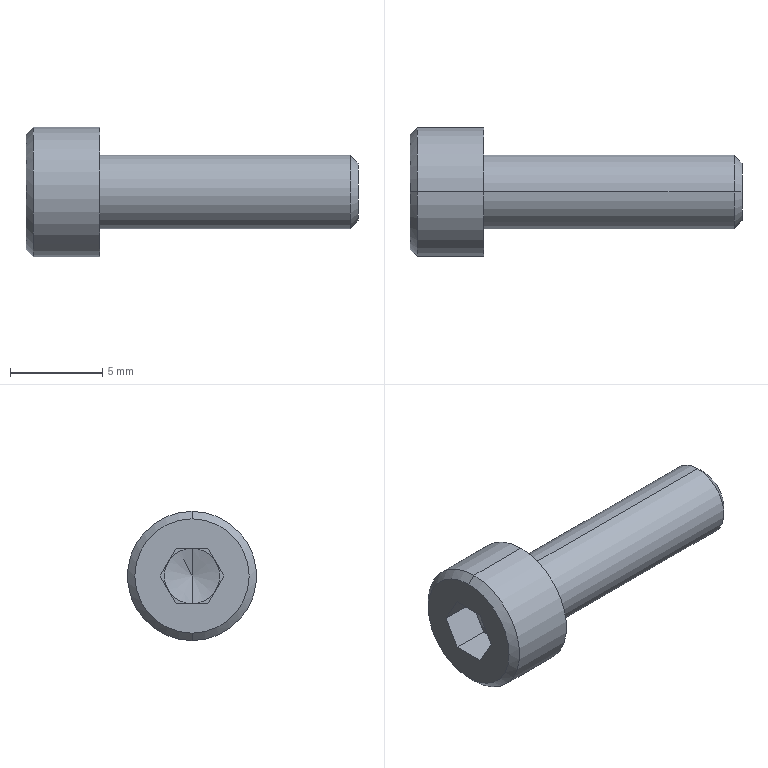Part | SolidWorks | features BaseBody 1 | 1 solid | 25 faces | box 18 x 7 x 7 mm | volume 310.563 mm3 | plane 15 | cone 6 | cylinder 4 | commonest cylinder face diameters 4 x2 7 x2
STEP:
#1=CARTESIAN_POINT('',(-4.,0.,3.1));
#2=VERTEX_POINT('',#1);
#3=CARTESIAN_POINT('',(-4.,0.,-3.1));
#4=VERTEX_POINT('',#3);
#5=CARTESIAN_POINT('',(-4.,0.,0.));
#6=DIRECTION('',(1.,0.,0.));
#7=DIRECTION('',(0.,0.,-1.));
#8=AXIS2_PLACEMENT_3D('',#5,#6,#7);
#9=CIRCLE('',#8,3.1);
#10=EDGE_CURVE('',#2,#4,#9,.T.);
#11=ORIENTED_EDGE('',*,*,#10,.F.);
#12=CARTESIAN_POINT('',(-4.,0.,0.));
#13=DIRECTION('',(1.,0.,0.));
#14=DIRECTION('',(0.,0.,-1.));
#15=AXIS2_PLACEMENT_3D('',#12,#13,#14);
#16=CIRCLE('',#15,3.1);
#17=EDGE_CURVE('',#4,#2,#16,.T.);
#18=ORIENTED_EDGE('',*,*,#17,.F.);
#19=EDGE_LOOP('',(#11,#18));
#20=FACE_OUTER_BOUND('',#19,.T.);
#21=CARTESIAN_POINT('',(-4.,-1.732,0.));
#22=VERTEX_POINT('',#21);
#23=CARTESIAN_POINT('',(-4.,-0.866,-1.5));
#24=VERTEX_POINT('',#23);
#25=CARTESIAN_POINT('',(-4.,-1.732,0.));
#26=DIRECTION('',(0.,0.5,-0.866));
#27=VECTOR('',#26,1000.);
#28=LINE('',#25,#27);
#29=EDGE_CURVE('',#22,#24,#28,.T.);
#30=ORIENTED_EDGE('',*,*,#29,.T.);
#31=CARTESIAN_POINT('',(-4.,0.866,-1.5));
#32=VERTEX_POINT('',#31);
#33=CARTESIAN_POINT('',(-4.,-0.866,-1.5));
#34=DIRECTION('',(0.,1.,0.));
#35=VECTOR('',#34,1000.);
#36=LINE('',#33,#35);
#37=EDGE_CURVE('',#24,#32,#36,.T.);
#38=ORIENTED_EDGE('',*,*,#37,.T.);
#39=CARTESIAN_POINT('',(-4.,1.732,0.));
#40=VERTEX_POINT('',#39);
#41=CARTESIAN_POINT('',(-4.,0.866,-1.5));
#42=DIRECTION('',(0.,0.5,0.866));
#43=VECTOR('',#42,1000.);
#44=LINE('',#41,#43);
#45=EDGE_CURVE('',#32,#40,#44,.T.);
#46=ORIENTED_EDGE('',*,*,#45,.T.);
#47=CARTESIAN_POINT('',(-4.,0.866,1.5));
#48=VERTEX_POINT('',#47);
#49=CARTESIAN_POINT('',(-4.,1.732,0.));
#50=DIRECTION('',(0.,-0.5,0.866));
#51=VECTOR('',#50,1000.);
#52=LINE('',#49,#51);
#53=EDGE_CURVE('',#40,#48,#52,.T.);
#54=ORIENTED_EDGE('',*,*,#53,.T.);
#55=CARTESIAN_POINT('',(-4.,-0.866,1.5));
#56=VERTEX_POINT('',#55);
#57=CARTESIAN_POINT('',(-4.,0.866,1.5));
#58=DIRECTION('',(0.,-1.,0.));
#59=VECTOR('',#58,1000.);
#60=LINE('',#57,#59);
#61=EDGE_CURVE('',#48,#56,#60,.T.);
#62=ORIENTED_EDGE('',*,*,#61,.T.);
#63=CARTESIAN_POINT('',(-4.,-0.866,1.5));
#64=DIRECTION('',(0.,-0.5,-0.866));
#65=VECTOR('',#64,1000.);
#66=LINE('',#63,#65);
#67=EDGE_CURVE('',#56,#22,#66,.T.);
#68=ORIENTED_EDGE('',*,*,#67,.T.);
#69=EDGE_LOOP('',(#30,#38,#46,#54,#62,#68));
#70=FACE_BOUND('',#69,.T.);
#71=CARTESIAN_POINT('',(-4.,0.,0.));
#72=DIRECTION('',(1.,0.,0.));
#73=DIRECTION('',(0.,0.,-1.));
#74=AXIS2_PLACEMENT_3D('',#71,#72,#73);
#75=PLANE('',#74);
#76=ADVANCED_FACE('',(#20,#70),#75,.F.);
#77=ORIENTED_EDGE('',*,*,#67,.F.);
#78=CARTESIAN_POINT('',(-2.,-0.866,1.5));
#79=VERTEX_POINT('',#78);
#80=CARTESIAN_POINT('',(-2.,-0.866,1.5));
#81=DIRECTION('',(-1.,0.,0.));
#82=VECTOR('',#81,1000.);
#83=LINE('',#80,#82);
#84=EDGE_CURVE('',#79,#56,#83,.T.);
#85=ORIENTED_EDGE('',*,*,#84,.F.);
#86=CARTESIAN_POINT('',(-2.,-1.299,0.75));
#87=VERTEX_POINT('',#86);
#88=CARTESIAN_POINT('',(-2.,-0.866,1.5));
#89=DIRECTION('',(0.,-0.5,-0.866));
#90=VECTOR('',#89,1000.);
#91=LINE('',#88,#90);
#92=EDGE_CURVE('',#79,#87,#91,.T.);
#93=ORIENTED_EDGE('',*,*,#92,.T.);
#94=CARTESIAN_POINT('',(-2.,-1.732,0.));
#95=VERTEX_POINT('',#94);
#96=CARTESIAN_POINT('',(-2.,-0.866,1.5));
#97=DIRECTION('',(0.,-0.5,-0.866));
#98=VECTOR('',#97,1000.);
#99=LINE('',#96,#98);
#100=EDGE_CURVE('',#87,#95,#99,.T.);
#101=ORIENTED_EDGE('',*,*,#100,.T.);
#102=CARTESIAN_POINT('',(-2.,-1.732,0.));
#103=DIRECTION('',(-1.,0.,0.));
#104=VECTOR('',#103,1000.);
#105=LINE('',#102,#104);
#106=EDGE_CURVE('',#95,#22,#105,.T.);
#107=ORIENTED_EDGE('',*,*,#106,.T.);
#108=EDGE_LOOP('',(#77,#85,#93,#101,#107));
#109=FACE_OUTER_BOUND('',#108,.T.);
#110=CARTESIAN_POINT('',(-2.,-0.866,1.5));
#111=DIRECTION('',(0.,0.866,-0.5));
#112=DIRECTION('',(0.,0.5,0.866));
#113=AXIS2_PLACEMENT_3D('',#110,#111,#112);
#114=PLANE('',#113);
#115=ADVANCED_FACE('',(#109),#114,.T.);
#116=ORIENTED_EDGE('',*,*,#29,.F.);
#117=ORIENTED_EDGE('',*,*,#106,.F.);
#118=CARTESIAN_POINT('',(-2.,-1.299,-0.75));
#119=VERTEX_POINT('',#118);
#120=CARTESIAN_POINT('',(-2.,-1.732,0.));
#121=DIRECTION('',(0.,0.5,-0.866));
#122=VECTOR('',#121,1000.);
#123=LINE('',#120,#122);
#124=EDGE_CURVE('',#95,#119,#123,.T.);
#125=ORIENTED_EDGE('',*,*,#124,.T.);
#126=CARTESIAN_POINT('',(-2.,-0.866,-1.5));
#127=VERTEX_POINT('',#126);
#128=CARTESIAN_POINT('',(-2.,-1.732,0.));
#129=DIRECTION('',(0.,0.5,-0.866));
#130=VECTOR('',#129,1000.);
#131=LINE('',#128,#130);
#132=EDGE_CURVE('',#119,#127,#131,.T.);
#133=ORIENTED_EDGE('',*,*,#132,.T.);
#134=CARTESIAN_POINT('',(-2.,-0.866,-1.5));
#135=DIRECTION('',(-1.,0.,0.));
#136=VECTOR('',#135,1000.);
#137=LINE('',#134,#136);
#138=EDGE_CURVE('',#127,#24,#137,.T.);
#139=ORIENTED_EDGE('',*,*,#138,.T.);
#140=EDGE_LOOP('',(#116,#117,#125,#133,#139));
#141=FACE_OUTER_BOUND('',#140,.T.);
#142=CARTESIAN_POINT('',(-2.,-1.732,0.));
#143=DIRECTION('',(0.,0.866,0.5));
#144=DIRECTION('',(0.,-0.5,0.866));
#145=AXIS2_PLACEMENT_3D('',#142,#143,#144);
#146=PLANE('',#145);
#147=ADVANCED_FACE('',(#141),#146,.T.);
#148=ORIENTED_EDGE('',*,*,#37,.F.);
#149=ORIENTED_EDGE('',*,*,#138,.F.);
#150=CARTESIAN_POINT('',(-2.,0.,-1.5));
#151=VERTEX_POINT('',#150);
#152=CARTESIAN_POINT('',(-2.,-0.866,-1.5));
#153=DIRECTION('',(0.,1.,0.));
#154=VECTOR('',#153,1000.);
#155=LINE('',#152,#154);
#156=EDGE_CURVE('',#127,#151,#155,.T.);
#157=ORIENTED_EDGE('',*,*,#156,.T.);
#158=CARTESIAN_POINT('',(-2.,0.866,-1.5));
#159=VERTEX_POINT('',#158);
#160=CARTESIAN_POINT('',(-2.,-0.866,-1.5));
#161=DIRECTION('',(0.,1.,0.));
#162=VECTOR('',#161,1000.);
#163=LINE('',#160,#162);
#164=EDGE_CURVE('',#151,#159,#163,.T.);
#165=ORIENTED_EDGE('',*,*,#164,.T.);
#166=CARTESIAN_POINT('',(-2.,0.866,-1.5));
#167=DIRECTION('',(-1.,0.,0.));
#168=VECTOR('',#167,1000.);
#169=LINE('',#166,#168);
#170=EDGE_CURVE('',#159,#32,#169,.T.);
#171=ORIENTED_EDGE('',*,*,#170,.T.);
#172=EDGE_LOOP('',(#148,#149,#157,#165,#171));
#173=FACE_OUTER_BOUND('',#172,.T.);
#174=CARTESIAN_POINT('',(-2.,-0.866,-1.5));
#175=DIRECTION('',(0.,0.,1.));
#176=DIRECTION('',(1.,0.,0.));
#177=AXIS2_PLACEMENT_3D('',#174,#175,#176);
#178=PLANE('',#177);
#179=ADVANCED_FACE('',(#173),#178,.T.);
#180=ORIENTED_EDGE('',*,*,#45,.F.);
#181=ORIENTED_EDGE('',*,*,#170,.F.);
#182=CARTESIAN_POINT('',(-2.,1.299,-0.75));
#183=VERTEX_POINT('',#182);
#184=CARTESIAN_POINT('',(-2.,0.866,-1.5));
#185=DIRECTION('',(0.,0.5,0.866));
#186=VECTOR('',#185,1000.);
#187=LINE('',#184,#186);
#188=EDGE_CURVE('',#159,#183,#187,.T.);
#189=ORIENTED_EDGE('',*,*,#188,.T.);
#190=CARTESIAN_POINT('',(-2.,1.732,0.));
#191=VERTEX_POINT('',#190);
#192=CARTESIAN_POINT('',(-2.,0.866,-1.5));
#193=DIRECTION('',(0.,0.5,0.866));
#194=VECTOR('',#193,1000.);
#195=LINE('',#192,#194);
#196=EDGE_CURVE('',#183,#191,#195,.T.);
#197=ORIENTED_EDGE('',*,*,#196,.T.);
#198=CARTESIAN_POINT('',(-2.,1.732,0.));
#199=DIRECTION('',(-1.,0.,0.));
#200=VECTOR('',#199,1000.);
#201=LINE('',#198,#200);
#202=EDGE_CURVE('',#191,#40,#201,.T.);
#203=ORIENTED_EDGE('',*,*,#202,.T.);
#204=EDGE_LOOP('',(#180,#181,#189,#197,#203));
#205=FACE_OUTER_BOUND('',#204,.T.);
#206=CARTESIAN_POINT('',(-2.,0.866,-1.5));
#207=DIRECTION('',(0.,-0.866,0.5));
#208=DIRECTION('',(0.,-0.5,-0.866));
#209=AXIS2_PLACEMENT_3D('',#206,#207,#208);
#210=PLANE('',#209);
#211=ADVANCED_FACE('',(#205),#210,.T.);
#212=ORIENTED_EDGE('',*,*,#53,.F.);
#213=ORIENTED_EDGE('',*,*,#202,.F.);
#214=CARTESIAN_POINT('',(-2.,1.299,0.75));
#215=VERTEX_POINT('',#214);
#216=CARTESIAN_POINT('',(-2.,1.732,0.));
#217=DIRECTION('',(0.,-0.5,0.866));
#218=VECTOR('',#217,1000.);
#219=LINE('',#216,#218);
#220=EDGE_CURVE('',#191,#215,#219,.T.);
#221=ORIENTED_EDGE('',*,*,#220,.T.);
#222=CARTESIAN_POINT('',(-2.,0.866,1.5));
#223=VERTEX_POINT('',#222);
#224=CARTESIAN_POINT('',(-2.,1.732,0.));
#225=DIRECTION('',(0.,-0.5,0.866));
#226=VECTOR('',#225,1000.);
#227=LINE('',#224,#226);
#228=EDGE_CURVE('',#215,#223,#227,.T.);
#229=ORIENTED_EDGE('',*,*,#228,.T.);
#230=CARTESIAN_POINT('',(-2.,0.866,1.5));
#231=DIRECTION('',(-1.,0.,0.));
#232=VECTOR('',#231,1000.);
#233=LINE('',#230,#232);
#234=EDGE_CURVE('',#223,#48,#233,.T.);
#235=ORIENTED_EDGE('',*,*,#234,.T.);
#236=EDGE_LOOP('',(#212,#213,#221,#229,#235));
#237=FACE_OUTER_BOUND('',#236,.T.);
#238=CARTESIAN_POINT('',(-2.,1.732,0.));
#239=DIRECTION('',(0.,-0.866,-0.5));
#240=DIRECTION('',(0.,0.5,-0.866));
#241=AXIS2_PLACEMENT_3D('',#238,#239,#240);
#242=PLANE('',#241);
#243=ADVANCED_FACE('',(#237),#242,.T.);
#244=ORIENTED_EDGE('',*,*,#61,.F.);
#245=ORIENTED_EDGE('',*,*,#234,.F.);
#246=CARTESIAN_POINT('',(-2.,0.,1.5));
#247=VERTEX_POINT('',#246);
#248=CARTESIAN_POINT('',(-2.,0.866,1.5));
#249=DIRECTION('',(0.,-1.,0.));
#250=VECTOR('',#249,1000.);
#251=LINE('',#248,#250);
#252=EDGE_CURVE('',#223,#247,#251,.T.);
#253=ORIENTED_EDGE('',*,*,#252,.T.);
#254=CARTESIAN_POINT('',(-2.,0.866,1.5));
#255=DIRECTION('',(0.,-1.,0.));
#256=VECTOR('',#255,1000.);
#257=LINE('',#254,#256);
#258=EDGE_CURVE('',#247,#79,#257,.T.);
#259=ORIENTED_EDGE('',*,*,#258,.T.);
#260=ORIENTED_EDGE('',*,*,#84,.T.);
#261=EDGE_LOOP('',(#244,#245,#253,#259,#260));
#262=FACE_OUTER_BOUND('',#261,.T.);
#263=CARTESIAN_POINT('',(-2.,0.866,1.5));
#264=DIRECTION('',(0.,0.,-1.));
#265=DIRECTION('',(-1.,0.,0.));
#266=AXIS2_PLACEMENT_3D('',#263,#264,#265);
#267=PLANE('',#266);
#268=ADVANCED_FACE('',(#262),#267,.T.);
#269=CARTESIAN_POINT('',(-2.,0.,0.));
#270=DIRECTION('',(1.,0.,0.));
#271=DIRECTION('',(0.,0.,-1.));
#272=AXIS2_PLACEMENT_3D('',#269,#270,#271);
#273=CIRCLE('',#272,1.5);
#274=EDGE_CURVE('',#247,#87,#273,.T.);
#275=ORIENTED_EDGE('',*,*,#274,.T.);
#276=ORIENTED_EDGE('',*,*,#92,.F.);
#277=ORIENTED_EDGE('',*,*,#258,.F.);
#278=EDGE_LOOP('',(#275,#276,#277));
#279=FACE_OUTER_BOUND('',#278,.T.);
#280=CARTESIAN_POINT('',(-2.,0.,0.));
#281=DIRECTION('',(1.,0.,0.));
#282=DIRECTION('',(0.,0.,-1.));
#283=AXIS2_PLACEMENT_3D('',#280,#281,#282);
#284=PLANE('',#283);
#285=ADVANCED_FACE('',(#279),#284,.F.);
#286=CARTESIAN_POINT('',(-1.598,0.,0.));
#287=VERTEX_POINT('',#286);
#288=CARTESIAN_POINT('',(-1.598,0.,0.));
#289=DIRECTION('',(-0.2588,0.,-0.9659));
#290=VECTOR('',#289,1000.);
#291=LINE('',#288,#290);
#292=EDGE_CURVE('',#287,#151,#291,.T.);
#293=ORIENTED_EDGE('',*,*,#292,.T.);
#294=CARTESIAN_POINT('',(-2.,0.,0.));
#295=DIRECTION('',(1.,0.,0.));
#296=DIRECTION('',(0.,0.,-1.));
#297=AXIS2_PLACEMENT_3D('',#294,#295,#296);
#298=CIRCLE('',#297,1.5);
#299=EDGE_CURVE('',#119,#151,#298,.T.);
#300=ORIENTED_EDGE('',*,*,#299,.F.);
#301=CARTESIAN_POINT('',(-2.,0.,0.));
#302=DIRECTION('',(1.,0.,0.));
#303=DIRECTION('',(0.,0.,-1.));
#304=AXIS2_PLACEMENT_3D('',#301,#302,#303);
#305=CIRCLE('',#304,1.5);
#306=EDGE_CURVE('',#87,#119,#305,.T.);
#307=ORIENTED_EDGE('',*,*,#306,.F.);
#308=ORIENTED_EDGE('',*,*,#274,.F.);
#309=CARTESIAN_POINT('',(-1.598,0.,0.));
#310=DIRECTION('',(-0.2588,0.,0.9659));
#311=VECTOR('',#310,1000.);
#312=LINE('',#309,#311);
#313=EDGE_CURVE('',#287,#247,#312,.T.);
#314=ORIENTED_EDGE('',*,*,#313,.F.);
#315=EDGE_LOOP('',(#293,#300,#307,#308,#314));
#316=FACE_OUTER_BOUND('',#315,.T.);
#317=CARTESIAN_POINT('',(-2.,0.,0.));
#318=DIRECTION('',(-1.,0.,0.));
#319=DIRECTION('',(0.,1.,0.));
#320=AXIS2_PLACEMENT_3D('',#317,#318,#319);
#321=CONICAL_SURFACE('',#320,1.5,1.309);
#322=ADVANCED_FACE('',(#316),#321,.F.);
#323=ORIENTED_EDGE('',*,*,#313,.T.);
#324=CARTESIAN_POINT('',(-2.,0.,0.));
#325=DIRECTION('',(1.,0.,0.));
#326=DIRECTION('',(0.,0.,-1.));
#327=AXIS2_PLACEMENT_3D('',#324,#325,#326);
#328=CIRCLE('',#327,1.5);
#329=EDGE_CURVE('',#215,#247,#328,.T.);
#330=ORIENTED_EDGE('',*,*,#329,.F.);
#331=CARTESIAN_POINT('',(-2.,0.,0.));
#332=DIRECTION('',(1.,0.,0.));
#333=DIRECTION('',(0.,0.,-1.));
#334=AXIS2_PLACEMENT_3D('',#331,#332,#333);
#335=CIRCLE('',#334,1.5);
#336=EDGE_CURVE('',#183,#215,#335,.T.);
#337=ORIENTED_EDGE('',*,*,#336,.F.);
#338=CARTESIAN_POINT('',(-2.,0.,0.));
#339=DIRECTION('',(1.,0.,0.));
#340=DIRECTION('',(0.,0.,-1.));
#341=AXIS2_PLACEMENT_3D('',#338,#339,#340);
#342=CIRCLE('',#341,1.5);
#343=EDGE_CURVE('',#151,#183,#342,.T.);
#344=ORIENTED_EDGE('',*,*,#343,.F.);
#345=ORIENTED_EDGE('',*,*,#292,.F.);
#346=EDGE_LOOP('',(#323,#330,#337,#344,#345));
#347=FACE_OUTER_BOUND('',#346,.T.);
#348=CARTESIAN_POINT('',(-2.,0.,0.));
#349=DIRECTION('',(-1.,0.,0.));
#350=DIRECTION('',(0.,-1.,0.));
#351=AXIS2_PLACEMENT_3D('',#348,#349,#350);
#352=CONICAL_SURFACE('',#351,1.5,1.309);
#353=ADVANCED_FACE('',(#347),#352,.F.);
#354=ORIENTED_EDGE('',*,*,#343,.T.);
#355=ORIENTED_EDGE('',*,*,#188,.F.);
#356=ORIENTED_EDGE('',*,*,#164,.F.);
#357=EDGE_LOOP('',(#354,#355,#356));
#358=FACE_OUTER_BOUND('',#357,.T.);
#359=CARTESIAN_POINT('',(-2.,0.,0.));
#360=DIRECTION('',(1.,0.,0.));
#361=DIRECTION('',(0.,0.,-1.));
#362=AXIS2_PLACEMENT_3D('',#359,#360,#361);
#363=PLANE('',#362);
#364=ADVANCED_FACE('',(#358),#363,.F.);
#365=ORIENTED_EDGE('',*,*,#196,.F.);
#366=ORIENTED_EDGE('',*,*,#336,.T.);
#367=ORIENTED_EDGE('',*,*,#220,.F.);
#368=EDGE_LOOP('',(#365,#366,#367));
#369=FACE_OUTER_BOUND('',#368,.T.);
#370=CARTESIAN_POINT('',(-2.,0.,0.));
#371=DIRECTION('',(1.,0.,0.));
#372=DIRECTION('',(0.,0.,-1.));
#373=AXIS2_PLACEMENT_3D('',#370,#371,#372);
#374=PLANE('',#373);
#375=ADVANCED_FACE('',(#369),#374,.F.);
#376=ORIENTED_EDGE('',*,*,#329,.T.);
#377=ORIENTED_EDGE('',*,*,#252,.F.);
#378=ORIENTED_EDGE('',*,*,#228,.F.);
#379=EDGE_LOOP('',(#376,#377,#378));
#380=FACE_OUTER_BOUND('',#379,.T.);
#381=CARTESIAN_POINT('',(-2.,0.,0.));
#382=DIRECTION('',(1.,0.,0.));
#383=DIRECTION('',(0.,0.,-1.));
#384=AXIS2_PLACEMENT_3D('',#381,#382,#383);
#385=PLANE('',#384);
#386=ADVANCED_FACE('',(#380),#385,.F.);
#387=ORIENTED_EDGE('',*,*,#306,.T.);
#388=ORIENTED_EDGE('',*,*,#124,.F.);
#389=ORIENTED_EDGE('',*,*,#100,.F.);
#390=EDGE_LOOP('',(#387,#388,#389));
#391=FACE_OUTER_BOUND('',#390,.T.);
#392=CARTESIAN_POINT('',(-2.,0.,0.));
#393=DIRECTION('',(1.,0.,0.));
#394=DIRECTION('',(0.,0.,-1.));
#395=AXIS2_PLACEMENT_3D('',#392,#393,#394);
#396=PLANE('',#395);
#397=ADVANCED_FACE('',(#391),#396,.F.);
#398=ORIENTED_EDGE('',*,*,#299,.T.);
#399=ORIENTED_EDGE('',*,*,#156,.F.);
#400=ORIENTED_EDGE('',*,*,#132,.F.);
#401=EDGE_LOOP('',(#398,#399,#400));
#402=FACE_OUTER_BOUND('',#401,.T.);
#403=CARTESIAN_POINT('',(-2.,0.,0.));
#404=DIRECTION('',(1.,0.,0.));
#405=DIRECTION('',(0.,0.,-1.));
#406=AXIS2_PLACEMENT_3D('',#403,#404,#405);
#407=PLANE('',#406);
#408=ADVANCED_FACE('',(#402),#407,.F.);
#409=CARTESIAN_POINT('',(-3.6,0.,3.5));
#410=VERTEX_POINT('',#409);
#411=CARTESIAN_POINT('',(-4.,0.,3.1));
#412=DIRECTION('',(0.7071,0.,0.7071));
#413=VECTOR('',#412,1000.);
#414=LINE('',#411,#413);
#415=EDGE_CURVE('',#2,#410,#414,.T.);
#416=ORIENTED_EDGE('',*,*,#415,.T.);
#417=CARTESIAN_POINT('',(-3.6,0.,-3.5));
#418=VERTEX_POINT('',#417);
#419=CARTESIAN_POINT('',(-3.6,0.,0.));
#420=DIRECTION('',(1.,0.,0.));
#421=DIRECTION('',(0.,0.,-1.));
#422=AXIS2_PLACEMENT_3D('',#419,#420,#421);
#423=CIRCLE('',#422,3.5);
#424=EDGE_CURVE('',#418,#410,#423,.T.);
#425=ORIENTED_EDGE('',*,*,#424,.F.);
#426=CARTESIAN_POINT('',(-4.,0.,-3.1));
#427=DIRECTION('',(0.7071,0.,-0.7071));
#428=VECTOR('',#427,1000.);
#429=LINE('',#426,#428);
#430=EDGE_CURVE('',#4,#418,#429,.T.);
#431=ORIENTED_EDGE('',*,*,#430,.F.);
#432=ORIENTED_EDGE('',*,*,#17,.T.);
#433=EDGE_LOOP('',(#416,#425,#431,#432));
#434=FACE_OUTER_BOUND('',#433,.T.);
#435=CARTESIAN_POINT('',(-4.,0.,0.));
#436=DIRECTION('',(1.,0.,0.));
#437=DIRECTION('',(0.,-1.,0.));
#438=AXIS2_PLACEMENT_3D('',#435,#436,#437);
#439=CONICAL_SURFACE('',#438,3.1,0.7854);
#440=ADVANCED_FACE('',(#434),#439,.T.);
#441=ORIENTED_EDGE('',*,*,#415,.F.);
#442=ORIENTED_EDGE('',*,*,#10,.T.);
#443=ORIENTED_EDGE('',*,*,#430,.T.);
#444=CARTESIAN_POINT('',(-3.6,0.,0.));
#445=DIRECTION('',(1.,0.,0.));
#446=DIRECTION('',(0.,0.,-1.));
#447=AXIS2_PLACEMENT_3D('',#444,#445,#446);
#448=CIRCLE('',#447,3.5);
#449=EDGE_CURVE('',#410,#418,#448,.T.);
#450=ORIENTED_EDGE('',*,*,#449,.F.);
#451=EDGE_LOOP('',(#441,#442,#443,#450));
#452=FACE_OUTER_BOUND('',#451,.T.);
#453=CARTESIAN_POINT('',(-4.,0.,0.));
#454=DIRECTION('',(1.,0.,0.));
#455=DIRECTION('',(0.,1.,0.));
#456=AXIS2_PLACEMENT_3D('',#453,#454,#455);
#457=CONICAL_SURFACE('',#456,3.1,0.7854);
#458=ADVANCED_FACE('',(#452),#457,.T.);
#459=CARTESIAN_POINT('',(0.,0.,3.5));
#460=VERTEX_POINT('',#459);
#461=CARTESIAN_POINT('',(-3.6,0.,3.5));
#462=DIRECTION('',(1.,0.,0.));
#463=VECTOR('',#462,1000.);
#464=LINE('',#461,#463);
#465=EDGE_CURVE('',#410,#460,#464,.T.);
#466=ORIENTED_EDGE('',*,*,#465,.F.);
#467=ORIENTED_EDGE('',*,*,#449,.T.);
#468=CARTESIAN_POINT('',(0.,0.,-3.5));
#469=VERTEX_POINT('',#468);
#470=CARTESIAN_POINT('',(-3.6,0.,-3.5));
#471=DIRECTION('',(1.,0.,0.));
#472=VECTOR('',#471,1000.);
#473=LINE('',#470,#472);
#474=EDGE_CURVE('',#418,#469,#473,.T.);
#475=ORIENTED_EDGE('',*,*,#474,.T.);
#476=CARTESIAN_POINT('',(0.,0.,0.));
#477=DIRECTION('',(1.,0.,0.));
#478=DIRECTION('',(0.,0.,-1.));
#479=AXIS2_PLACEMENT_3D('',#476,#477,#478);
#480=CIRCLE('',#479,3.5);
#481=EDGE_CURVE('',#460,#469,#480,.T.);
#482=ORIENTED_EDGE('',*,*,#481,.F.);
#483=EDGE_LOOP('',(#466,#467,#475,#482));
#484=FACE_OUTER_BOUND('',#483,.T.);
#485=CARTESIAN_POINT('',(14.,0.,0.));
#486=DIRECTION('',(1.,0.,0.));
#487=DIRECTION('',(0.,1.,0.));
#488=AXIS2_PLACEMENT_3D('',#485,#486,#487);
#489=CYLINDRICAL_SURFACE('',#488,3.5);
#490=ADVANCED_FACE('',(#484),#489,.T.);
#491=CARTESIAN_POINT('',(0.,0.,2.));
#492=VERTEX_POINT('',#491);
#493=CARTESIAN_POINT('',(0.,0.,-2.));
#494=VERTEX_POINT('',#493);
#495=CARTESIAN_POINT('',(0.,0.,0.));
#496=DIRECTION('',(1.,0.,0.));
#497=DIRECTION('',(0.,0.,-1.));
#498=AXIS2_PLACEMENT_3D('',#495,#496,#497);
#499=CIRCLE('',#498,2.);
#500=EDGE_CURVE('',#492,#494,#499,.T.);
#501=ORIENTED_EDGE('',*,*,#500,.F.);
#502=CARTESIAN_POINT('',(0.,0.,0.));
#503=DIRECTION('',(1.,0.,0.));
#504=DIRECTION('',(0.,0.,-1.));
#505=AXIS2_PLACEMENT_3D('',#502,#503,#504);
#506=CIRCLE('',#505,2.);
#507=EDGE_CURVE('',#494,#492,#506,.T.);
#508=ORIENTED_EDGE('',*,*,#507,.F.);
#509=EDGE_LOOP('',(#501,#508));
#510=FACE_BOUND('',#509,.T.);
#511=CARTESIAN_POINT('',(0.,0.,0.));
#512=DIRECTION('',(1.,0.,0.));
#513=DIRECTION('',(0.,0.,-1.));
#514=AXIS2_PLACEMENT_3D('',#511,#512,#513);
#515=CIRCLE('',#514,3.5);
#516=EDGE_CURVE('',#469,#460,#515,.T.);
#517=ORIENTED_EDGE('',*,*,#516,.T.);
#518=ORIENTED_EDGE('',*,*,#481,.T.);
#519=EDGE_LOOP('',(#517,#518));
#520=FACE_OUTER_BOUND('',#519,.T.);
#521=CARTESIAN_POINT('',(0.,3.5,0.));
#522=DIRECTION('',(-1.,0.,0.));
#523=DIRECTION('',(0.,0.,1.));
#524=AXIS2_PLACEMENT_3D('',#521,#522,#523);
#525=PLANE('',#524);
#526=ADVANCED_FACE('',(#510,#520),#525,.F.);
#527=ORIENTED_EDGE('',*,*,#465,.T.);
#528=ORIENTED_EDGE('',*,*,#516,.F.);
#529=ORIENTED_EDGE('',*,*,#474,.F.);
#530=ORIENTED_EDGE('',*,*,#424,.T.);
#531=EDGE_LOOP('',(#527,#528,#529,#530));
#532=FACE_OUTER_BOUND('',#531,.T.);
#533=CARTESIAN_POINT('',(14.,0.,0.));
#534=DIRECTION('',(1.,0.,0.));
#535=DIRECTION('',(0.,-1.,0.));
#536=AXIS2_PLACEMENT_3D('',#533,#534,#535);
#537=CYLINDRICAL_SURFACE('',#536,3.5);
#538=ADVANCED_FACE('',(#532),#537,.T.);
#539=CARTESIAN_POINT('',(13.57,0.,2.));
#540=VERTEX_POINT('',#539);
#541=CARTESIAN_POINT('',(0.,0.,2.));
#542=DIRECTION('',(1.,0.,0.));
#543=VECTOR('',#542,1000.);
#544=LINE('',#541,#543);
#545=EDGE_CURVE('',#492,#540,#544,.T.);
#546=ORIENTED_EDGE('',*,*,#545,.T.);
#547=CARTESIAN_POINT('',(13.57,0.,-2.));
#548=VERTEX_POINT('',#547);
#549=CARTESIAN_POINT('',(13.57,0.,0.));
#550=DIRECTION('',(1.,0.,0.));
#551=DIRECTION('',(0.,0.,-1.));
#552=AXIS2_PLACEMENT_3D('',#549,#550,#551);
#553=CIRCLE('',#552,2.);
#554=EDGE_CURVE('',#548,#540,#553,.T.);
#555=ORIENTED_EDGE('',*,*,#554,.F.);
#556=CARTESIAN_POINT('',(0.,0.,-2.));
#557=DIRECTION('',(1.,0.,0.));
#558=VECTOR('',#557,1000.);
#559=LINE('',#556,#558);
#560=EDGE_CURVE('',#494,#548,#559,.T.);
#561=ORIENTED_EDGE('',*,*,#560,.F.);
#562=ORIENTED_EDGE('',*,*,#507,.T.);
#563=EDGE_LOOP('',(#546,#555,#561,#562));
#564=FACE_OUTER_BOUND('',#563,.T.);
#565=CARTESIAN_POINT('',(14.,0.,0.));
#566=DIRECTION('',(1.,0.,0.));
#567=DIRECTION('',(0.,-1.,0.));
#568=AXIS2_PLACEMENT_3D('',#565,#566,#567);
#569=CYLINDRICAL_SURFACE('',#568,2.);
#570=ADVANCED_FACE('',(#564),#569,.T.);
#571=ORIENTED_EDGE('',*,*,#545,.F.);
#572=ORIENTED_EDGE('',*,*,#500,.T.);
#573=ORIENTED_EDGE('',*,*,#560,.T.);
#574=CARTESIAN_POINT('',(13.57,0.,0.));
#575=DIRECTION('',(1.,0.,0.));
#576=DIRECTION('',(0.,0.,-1.));
#577=AXIS2_PLACEMENT_3D('',#574,#575,#576);
#578=CIRCLE('',#577,2.);
#579=EDGE_CURVE('',#540,#548,#578,.T.);
#580=ORIENTED_EDGE('',*,*,#579,.F.);
#581=EDGE_LOOP('',(#571,#572,#573,#580));
#582=FACE_OUTER_BOUND('',#581,.T.);
#583=CARTESIAN_POINT('',(14.,0.,0.));
#584=DIRECTION('',(1.,0.,0.));
#585=DIRECTION('',(0.,1.,0.));
#586=AXIS2_PLACEMENT_3D('',#583,#584,#585);
#587=CYLINDRICAL_SURFACE('',#586,2.);
#588=ADVANCED_FACE('',(#582),#587,.T.);
#589=CARTESIAN_POINT('',(14.,0.,-1.571));
#590=VERTEX_POINT('',#589);
#591=CARTESIAN_POINT('',(14.,0.,-1.57));
#592=DIRECTION('',(-0.7071,0.,-0.7071));
#593=VECTOR('',#592,1000.);
#594=LINE('',#591,#593);
#595=EDGE_CURVE('',#590,#548,#594,.T.);
#596=ORIENTED_EDGE('',*,*,#595,.F.);
#597=CARTESIAN_POINT('',(14.,0.,1.57));
#598=VERTEX_POINT('',#597);
#599=CARTESIAN_POINT('',(14.,0.,0.));
#600=DIRECTION('',(1.,0.,0.));
#601=DIRECTION('',(0.,0.,-1.));
#602=AXIS2_PLACEMENT_3D('',#599,#600,#601);
#603=CIRCLE('',#602,1.571);
#604=EDGE_CURVE('',#598,#590,#603,.T.);
#605=ORIENTED_EDGE('',*,*,#604,.F.);
#606=CARTESIAN_POINT('',(14.,0.,1.57));
#607=DIRECTION('',(-0.7071,0.,0.7071));
#608=VECTOR('',#607,1000.);
#609=LINE('',#606,#608);
#610=EDGE_CURVE('',#598,#540,#609,.T.);
#611=ORIENTED_EDGE('',*,*,#610,.T.);
#612=ORIENTED_EDGE('',*,*,#579,.T.);
#613=EDGE_LOOP('',(#596,#605,#611,#612));
#614=FACE_OUTER_BOUND('',#613,.T.);
#615=CARTESIAN_POINT('',(13.57,0.,0.));
#616=DIRECTION('',(-1.,0.,0.));
#617=DIRECTION('',(0.,1.,0.));
#618=AXIS2_PLACEMENT_3D('',#615,#616,#617);
#619=CONICAL_SURFACE('',#618,2.,0.7854);
#620=ADVANCED_FACE('',(#614),#619,.T.);
#621=ORIENTED_EDGE('',*,*,#595,.T.);
#622=ORIENTED_EDGE('',*,*,#554,.T.);
#623=ORIENTED_EDGE('',*,*,#610,.F.);
#624=CARTESIAN_POINT('',(14.,0.,0.));
#625=DIRECTION('',(1.,0.,0.));
#626=DIRECTION('',(0.,0.,-1.));
#627=AXIS2_PLACEMENT_3D('',#624,#625,#626);
#628=CIRCLE('',#627,1.571);
#629=EDGE_CURVE('',#590,#598,#628,.T.);
#630=ORIENTED_EDGE('',*,*,#629,.F.);
#631=EDGE_LOOP('',(#621,#622,#623,#630));
#632=FACE_OUTER_BOUND('',#631,.T.);
#633=CARTESIAN_POINT('',(13.57,0.,0.));
#634=DIRECTION('',(-1.,0.,0.));
#635=DIRECTION('',(0.,-1.,0.));
#636=AXIS2_PLACEMENT_3D('',#633,#634,#635);
#637=CONICAL_SURFACE('',#636,2.,0.7854);
#638=ADVANCED_FACE('',(#632),#637,.T.);
#639=ORIENTED_EDGE('',*,*,#629,.T.);
#640=ORIENTED_EDGE('',*,*,#604,.T.);
#641=EDGE_LOOP('',(#639,#640));
#642=FACE_OUTER_BOUND('',#641,.T.);
#643=CARTESIAN_POINT('',(14.,1.571,0.));
#644=DIRECTION('',(-1.,0.,0.));
#645=DIRECTION('',(0.,0.,1.));
#646=AXIS2_PLACEMENT_3D('',#643,#644,#645);
#647=PLANE('',#646);
#648=ADVANCED_FACE('',(#642),#647,.F.);
#649=CLOSED_SHELL('',(#76,#115,#147,#179,#211,#243,#268,#285,#322,#353,#364,#375,#386,#397,#408,#440,#458,#490,#526,#538,#570,#588,#620,#638,#648));
#650=MANIFOLD_SOLID_BREP('',#649);
#651=CARTESIAN_POINT('',(0.,0.,0.));
#652=DIRECTION('',(0.,0.,1.));
#653=DIRECTION('',(1.,0.,0.));
#654=AXIS2_PLACEMENT_3D('',#651,#652,#653);
#655=(LENGTH_UNIT()NAMED_UNIT(*)SI_UNIT(.MILLI.,.METRE.));
#656=UNCERTAINTY_MEASURE_WITH_UNIT(LENGTH_MEASURE(0.00001),#655,'','');
#657=(NAMED_UNIT(*)PLANE_ANGLE_UNIT()SI_UNIT($,.RADIAN.));
#658=(NAMED_UNIT(*)SI_UNIT($,.STERADIAN.)SOLID_ANGLE_UNIT());
#659=(GEOMETRIC_REPRESENTATION_CONTEXT(3)GLOBAL_UNCERTAINTY_ASSIGNED_CONTEXT((#656))GLOBAL_UNIT_ASSIGNED_CONTEXT((#655,#657,#658))REPRESENTATION_CONTEXT('',''));
#660=ADVANCED_BREP_SHAPE_REPRESENTATION('',(#650,#654),#659);